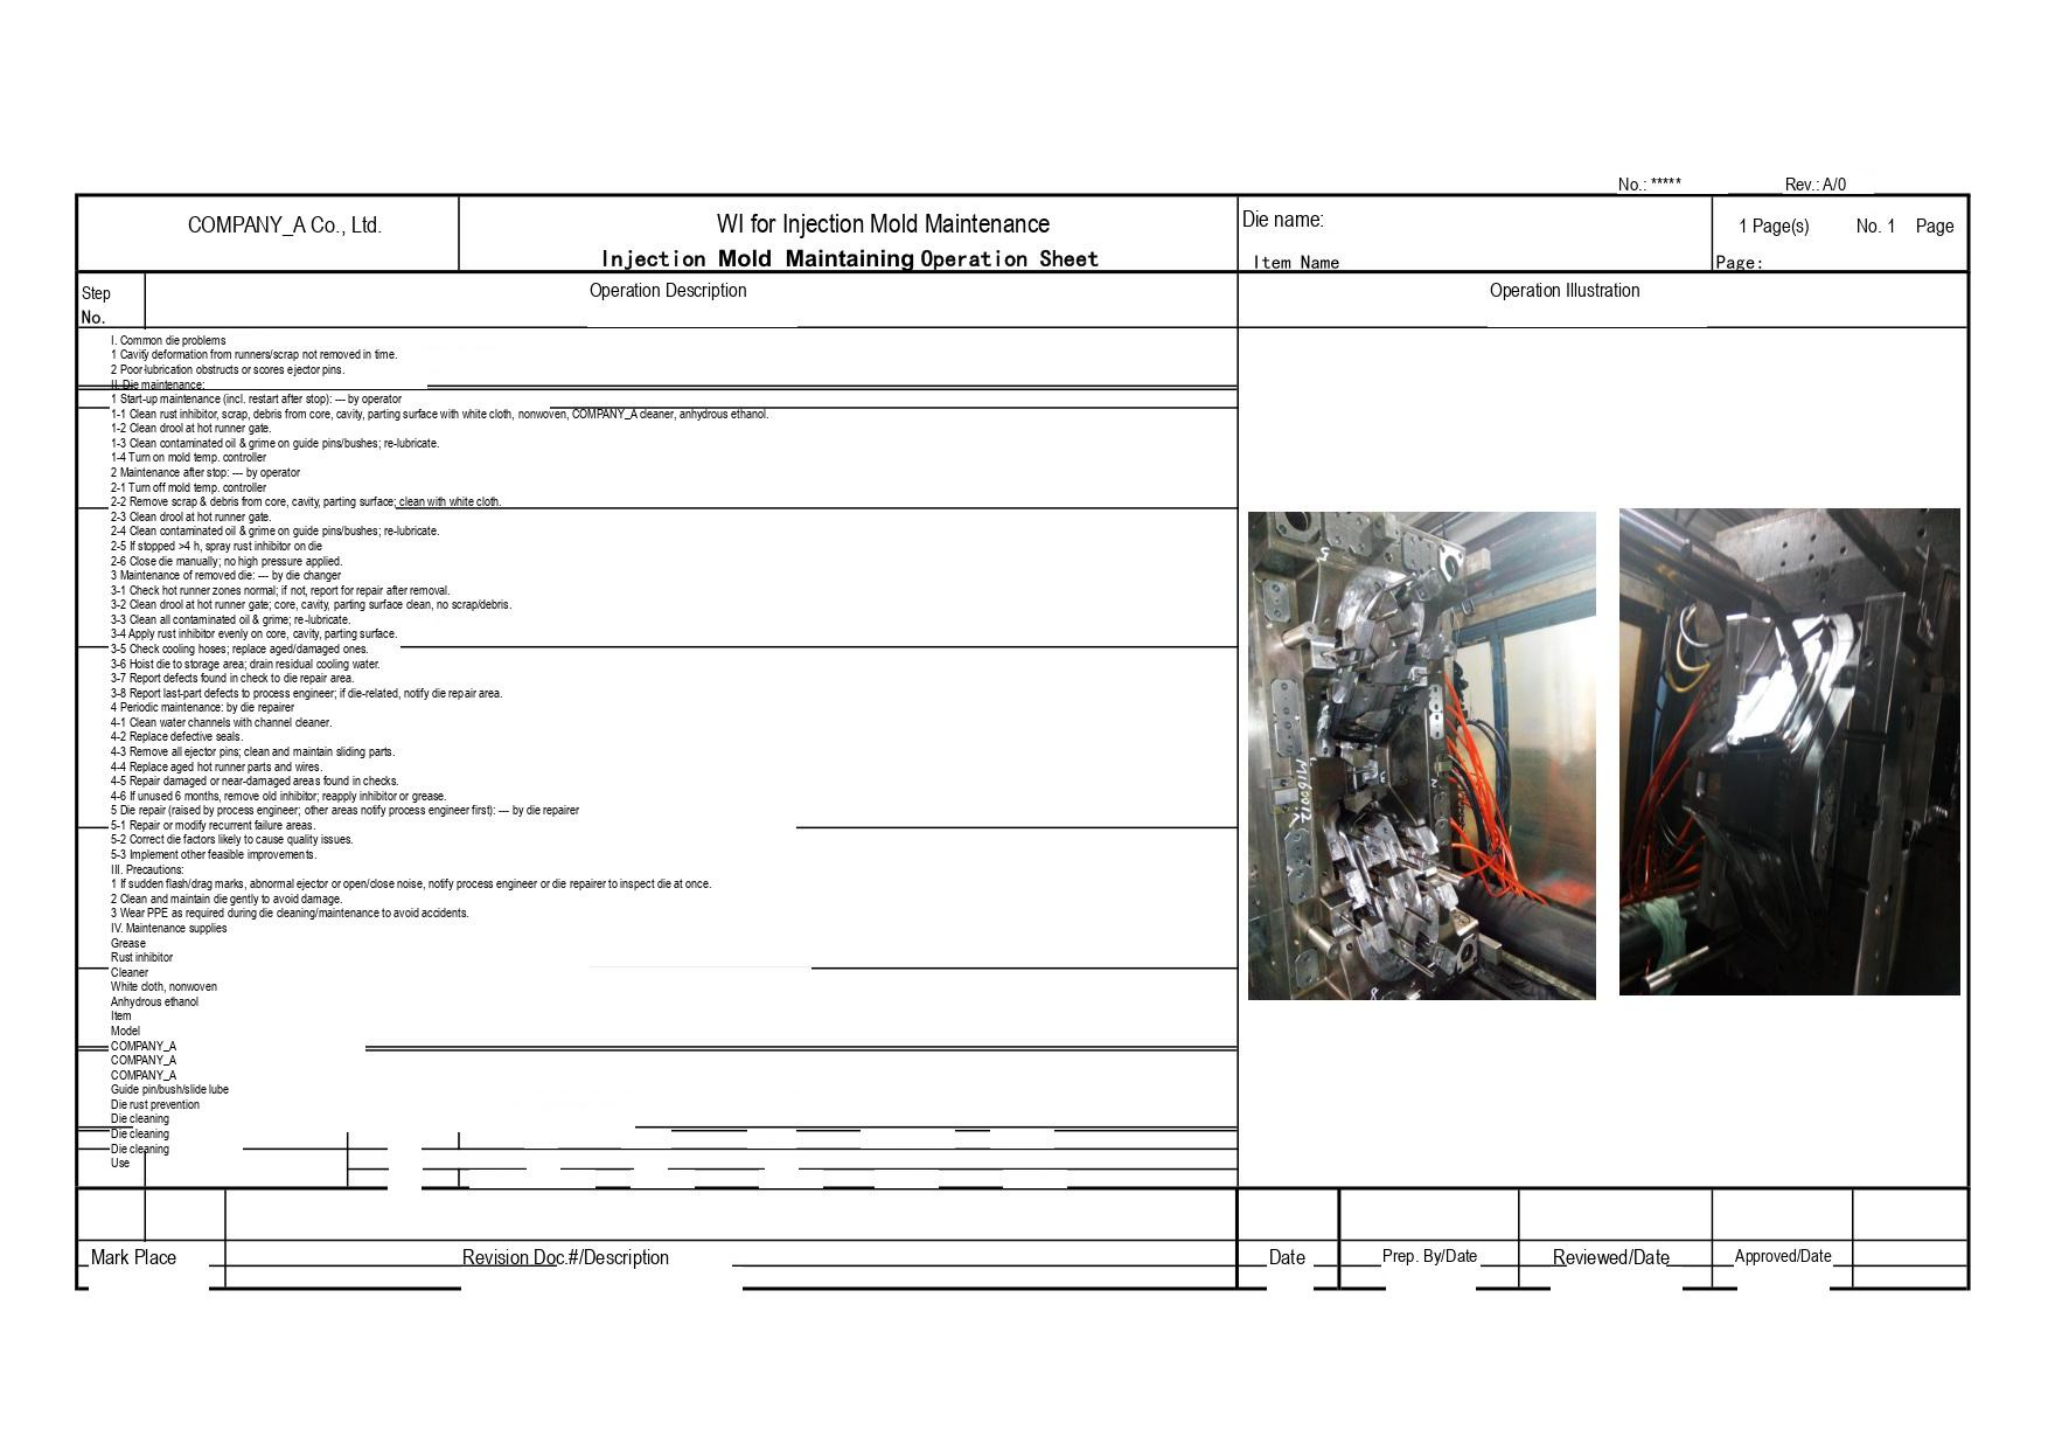No.: ***** Rev.: A/0

| COMPANY_A Co., Ltd. | WI for Injection Mold Maintenance<br>Injection Mold Maintaining Operation Sheet | Die name:<br>Item Name | 1 Page(s) No. 1 Page<br>Page: |
|---|---|---|---|

| Step No. | Operation Description | Operation Illustration |
|---|---|---|

I. Common die problems
1 Cavity deformation from runners/scrap not removed in time.
2 Poor lubrication obstructs or scores ejector pins.
II. Die maintenance:
1 Start-up maintenance (incl. restart after stop): — by operator
1-1 Clean rust inhibitor, scrap, debris from core, cavity, parting surface with white cloth, nonwoven, COMPANY_A cleaner, anhydrous ethanol.
1-2 Clean drool at hot runner gate.
1-3 Clean contaminated oil & grime on guide pins/bushes; re-lubricate.
1-4 Turn on mold temp. controller
2 Maintenance after stop: — by operator
2-1 Turn off mold temp. controller
2-2 Remove scrap & debris from core, cavity, parting surface; clean with white cloth.
2-3 Clean drool at hot runner gate.
2-4 Clean contaminated oil & grime on guide pins/bushes; re-lubricate.
2-5 If stopped >4 h, spray rust inhibitor on die
2-6 Close die manually; no high pressure applied.
3 Maintenance of removed die: — by die changer
3-1 Check hot runner zones normal; if not, report for repair after removal.
3-2 Clean drool at hot runner gate; core, cavity, parting surface clean, no scrap/debris.
3-3 Clean all contaminated oil & grime; re-lubricate.
3-4 Apply rust inhibitor evenly on core, cavity, parting surface.
3-5 Check cooling hoses; replace aged/damaged ones.
3-6 Hoist die to storage area; drain residual cooling water.
3-7 Report defects found in check to die repair area.
3-8 Report last-part defects to process engineer; if die-related, notify die repair area.
4 Periodic maintenance: by die repairer
4-1 Clean water channels with channel cleaner.
4-2 Replace defective seals.
4-3 Remove all ejector pins; clean and maintain sliding parts.
4-4 Replace aged hot runner parts and wires.
4-5 Repair damaged or near-damaged areas found in checks.
4-6 If unused 6 months, remove old inhibitor; reapply inhibitor or grease.
5 Die repair (raised by process engineer; other areas notify process engineer first): — by die repairer
5-1 Repair or modify recurrent failure areas.
5-2 Correct die factors likely to cause quality issues.
5-3 Implement other feasible improvements.
III. Precautions:
1 If sudden flash/drag marks, abnormal ejector or open/close noise, notify process engineer or die repairer to inspect die at once.
2 Clean and maintain die gently to avoid damage.
3 Wear PPE as required during die cleaning/maintenance to avoid accidents.
IV. Maintenance supplies
Grease
Rust inhibitor
Cleaner
White cloth, nonwoven
Anhydrous ethanol
Item
Model
COMPANY_A
COMPANY_A
COMPANY_A
Guide pin/bush/slide lube
Die rust prevention
Die cleaning
Die cleaning
Die cleaning
Use

| Mark | Place | Revision Doc.#/Description | Date | Prep. By/Date | Reviewed/Date | Approved/Date |
|---|---|---|---|---|---|---|